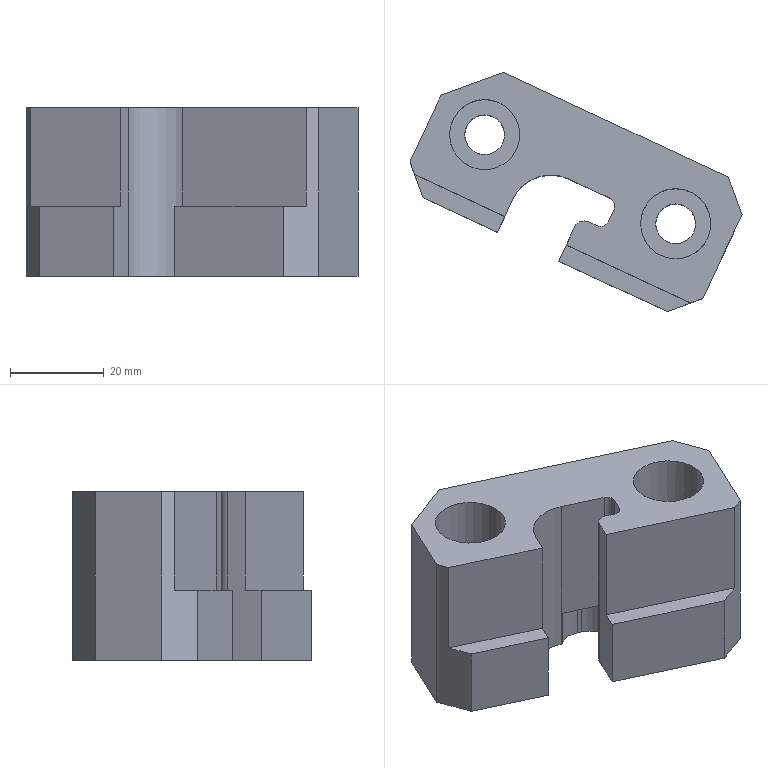Part | STEP file | gslz 2016.10.28-13_id1674_x_t | 1 solid | 34 faces | box 70.882 x 51.053 x 36 mm | volume 51884 mm3 | plane 24 | cylinder 10 | commonest cylinder face diameters 3.5 x2 8.5 x2 10 x2 15 x2 4.5 x1 18 x1